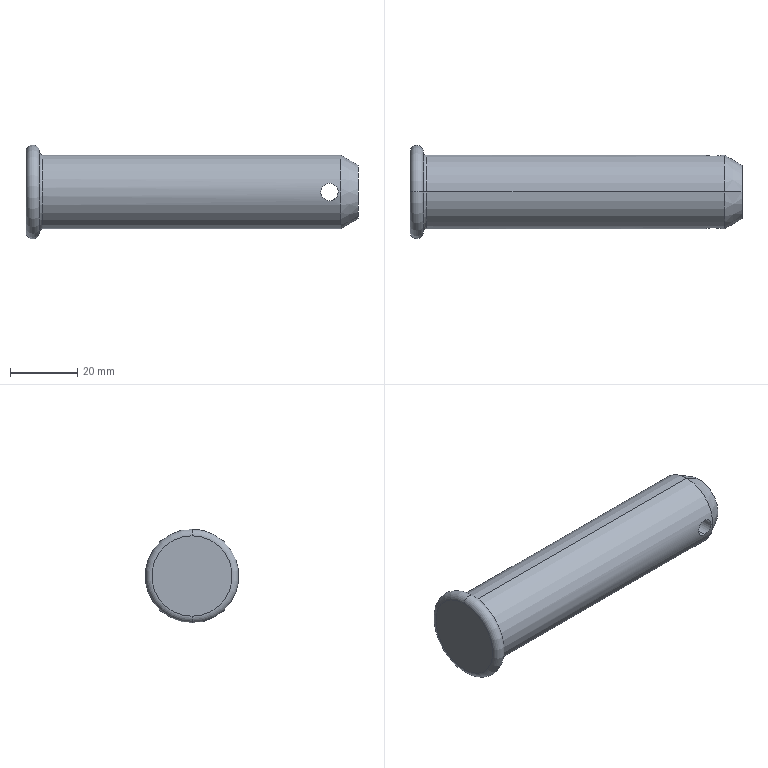Part | SolidWorks | features Chamfer 1, Cut 1, Fillet 1, Revolution 1 | 1 solid | 12 faces | box 99 x 28 x 28 mm | volume 37494 mm3 | cylinder 4 | torus 4 | cone 2 | plane 2 | commonest cylinder face diameters 5.18 x2 22 x2
STEP:
#1=CARTESIAN_POINT('',(90.5,-10.691,-2.59));
#2=VERTEX_POINT('',#1);
#3=CARTESIAN_POINT('',(90.5,-10.691,2.59));
#4=VERTEX_POINT('',#3);
#5=CARTESIAN_POINT('',(90.5,-10.691,-2.59));
#6=CARTESIAN_POINT('',(90.161,-10.691,-2.59));
#7=CARTESIAN_POINT('',(89.819,-10.708,-2.522));
#8=CARTESIAN_POINT('',(89.352,-10.751,-2.328));
#9=CARTESIAN_POINT('',(89.2,-10.769,-2.247));
#10=CARTESIAN_POINT('',(88.919,-10.806,-2.058));
#11=CARTESIAN_POINT('',(88.789,-10.826,-1.952));
#12=CARTESIAN_POINT('',(88.55,-10.866,-1.713));
#13=CARTESIAN_POINT('',(88.441,-10.887,-1.58));
#14=CARTESIAN_POINT('',(88.254,-10.924,-1.3));
#15=CARTESIAN_POINT('',(88.174,-10.941,-1.152));
#16=CARTESIAN_POINT('',(87.978,-10.984,-0.6798));
#17=CARTESIAN_POINT('',(87.91,-11.,-0.3427));
#18=CARTESIAN_POINT('',(87.91,-11.,0.1699));
#19=CARTESIAN_POINT('',(87.927,-10.996,0.3384));
#20=CARTESIAN_POINT('',(87.993,-10.981,0.6709));
#21=CARTESIAN_POINT('',(88.043,-10.969,0.8362));
#22=CARTESIAN_POINT('',(88.173,-10.941,1.149));
#23=CARTESIAN_POINT('',(88.252,-10.924,1.297));
#24=CARTESIAN_POINT('',(88.441,-10.887,1.58));
#25=CARTESIAN_POINT('',(88.549,-10.867,1.711));
#26=CARTESIAN_POINT('',(88.905,-10.806,2.068));
#27=CARTESIAN_POINT('',(89.193,-10.766,2.261));
#28=CARTESIAN_POINT('',(89.66,-10.723,2.456));
#29=CARTESIAN_POINT('',(89.825,-10.711,2.506));
#30=CARTESIAN_POINT('',(90.159,-10.695,2.573));
#31=CARTESIAN_POINT('',(90.328,-10.691,2.59));
#32=CARTESIAN_POINT('',(90.5,-10.691,2.59));
#33=B_SPLINE_CURVE_WITH_KNOTS('',3,(#5,#6,#7,#8,#9,#10,#11,#12,#13,#14,#15,#16,#17,#18,#19,#20,#21,#22,#23,#24,#25,#26,#27,#28,#29,#30,#31,#32),.UNSPECIFIED.,.F.,.F.,(4,2,2,2,2,2,2,2,2,2,2,2,2,4),(0.008126,0.009142,0.009649,0.01016,0.01066,0.01117,0.01219,0.0127,0.0132,0.01371,0.01422,0.01523,0.01574,0.01625),.UNSPECIFIED.);
#34=EDGE_CURVE('',#2,#4,#33,.T.);
#35=ORIENTED_EDGE('',*,*,#34,.F.);
#36=CARTESIAN_POINT('',(90.5,10.691,-2.59));
#37=VERTEX_POINT('',#36);
#38=CARTESIAN_POINT('',(90.5,-500.,-2.59));
#39=DIRECTION('',(0.,1.,0.));
#40=VECTOR('',#39,1000.);
#41=LINE('',#38,#40);
#42=EDGE_CURVE('',#2,#37,#41,.T.);
#43=ORIENTED_EDGE('',*,*,#42,.T.);
#44=CARTESIAN_POINT('',(90.5,10.691,2.59));
#45=VERTEX_POINT('',#44);
#46=CARTESIAN_POINT('',(90.5,10.691,2.59));
#47=CARTESIAN_POINT('',(90.328,10.691,2.59));
#48=CARTESIAN_POINT('',(90.159,10.695,2.573));
#49=CARTESIAN_POINT('',(89.828,10.711,2.507));
#50=CARTESIAN_POINT('',(89.663,10.722,2.457));
#51=CARTESIAN_POINT('',(89.349,10.751,2.327));
#52=CARTESIAN_POINT('',(89.201,10.768,2.247));
#53=CARTESIAN_POINT('',(88.92,10.806,2.059));
#54=CARTESIAN_POINT('',(88.787,10.826,1.95));
#55=CARTESIAN_POINT('',(88.43,10.887,1.593));
#56=CARTESIAN_POINT('',(88.237,10.927,1.305));
#57=CARTESIAN_POINT('',(88.043,10.969,0.8377));
#58=CARTESIAN_POINT('',(87.993,10.981,0.6738));
#59=CARTESIAN_POINT('',(87.927,10.996,0.3391));
#60=CARTESIAN_POINT('',(87.91,11.,0.1707));
#61=CARTESIAN_POINT('',(87.91,11.,-0.1686));
#62=CARTESIAN_POINT('',(87.927,10.996,-0.3409));
#63=CARTESIAN_POINT('',(87.993,10.981,-0.6736));
#64=CARTESIAN_POINT('',(88.043,10.969,-0.8353));
#65=CARTESIAN_POINT('',(88.238,10.927,-1.307));
#66=CARTESIAN_POINT('',(88.429,10.887,-1.592));
#67=CARTESIAN_POINT('',(88.789,10.826,-1.952));
#68=CARTESIAN_POINT('',(88.919,10.806,-2.059));
#69=CARTESIAN_POINT('',(89.199,10.769,-2.246));
#70=CARTESIAN_POINT('',(89.351,10.751,-2.327));
#71=CARTESIAN_POINT('',(89.664,10.722,-2.457));
#72=CARTESIAN_POINT('',(89.825,10.711,-2.506));
#73=CARTESIAN_POINT('',(90.159,10.695,-2.573));
#74=CARTESIAN_POINT('',(90.331,10.691,-2.59));
#75=CARTESIAN_POINT('',(90.5,10.691,-2.59));
#76=B_SPLINE_CURVE_WITH_KNOTS('',3,(#46,#47,#48,#49,#50,#51,#52,#53,#54,#55,#56,#57,#58,#59,#60,#61,#62,#63,#64,#65,#66,#67,#68,#69,#70,#71,#72,#73,#74,#75),.UNSPECIFIED.,.F.,.F.,(4,2,2,2,2,2,2,2,2,2,2,2,2,2,4),(0.,0.0005079,0.001016,0.001524,0.002032,0.003047,0.003555,0.004063,0.004571,0.005079,0.006095,0.006602,0.00711,0.007618,0.008126),.UNSPECIFIED.);
#77=EDGE_CURVE('',#45,#37,#76,.T.);
#78=ORIENTED_EDGE('',*,*,#77,.F.);
#79=CARTESIAN_POINT('',(90.5,-500.,2.59));
#80=DIRECTION('',(0.,1.,0.));
#81=VECTOR('',#80,1000.);
#82=LINE('',#79,#81);
#83=EDGE_CURVE('',#4,#45,#82,.T.);
#84=ORIENTED_EDGE('',*,*,#83,.F.);
#85=EDGE_LOOP('',(#35,#43,#78,#84));
#86=FACE_OUTER_BOUND('',#85,.T.);
#87=CARTESIAN_POINT('',(90.5,-500.,0.));
#88=DIRECTION('',(0.,1.,0.));
#89=DIRECTION('',(0.,0.,1.));
#90=AXIS2_PLACEMENT_3D('',#87,#88,#89);
#91=CYLINDRICAL_SURFACE('',#90,2.59);
#92=ADVANCED_FACE('',(#86),#91,.F.);
#93=CARTESIAN_POINT('',(99.,0.,-8.));
#94=VERTEX_POINT('',#93);
#95=CARTESIAN_POINT('',(99.,0.,8.));
#96=VERTEX_POINT('',#95);
#97=CARTESIAN_POINT('',(99.,0.,0.));
#98=DIRECTION('',(1.,0.,0.));
#99=DIRECTION('',(0.,0.,1.));
#100=AXIS2_PLACEMENT_3D('',#97,#98,#99);
#101=CIRCLE('',#100,8.);
#102=EDGE_CURVE('',#94,#96,#101,.T.);
#103=ORIENTED_EDGE('',*,*,#102,.F.);
#104=CARTESIAN_POINT('',(93.804,0.,-11.));
#105=VERTEX_POINT('',#104);
#106=CARTESIAN_POINT('',(93.804,0.,-11.));
#107=DIRECTION('',(-0.866,0.,-0.5));
#108=VECTOR('',#107,1000.);
#109=LINE('',#106,#108);
#110=EDGE_CURVE('',#94,#105,#109,.T.);
#111=ORIENTED_EDGE('',*,*,#110,.T.);
#112=CARTESIAN_POINT('',(93.804,0.,11.));
#113=VERTEX_POINT('',#112);
#114=CARTESIAN_POINT('',(93.804,0.,0.));
#115=DIRECTION('',(-1.,0.,0.));
#116=DIRECTION('',(0.,0.,1.));
#117=AXIS2_PLACEMENT_3D('',#114,#115,#116);
#118=CIRCLE('',#117,11.);
#119=EDGE_CURVE('',#113,#105,#118,.T.);
#120=ORIENTED_EDGE('',*,*,#119,.F.);
#121=CARTESIAN_POINT('',(93.804,0.,11.));
#122=DIRECTION('',(-0.866,0.,0.5));
#123=VECTOR('',#122,1000.);
#124=LINE('',#121,#123);
#125=EDGE_CURVE('',#96,#113,#124,.T.);
#126=ORIENTED_EDGE('',*,*,#125,.F.);
#127=EDGE_LOOP('',(#103,#111,#120,#126));
#128=FACE_OUTER_BOUND('',#127,.T.);
#129=CARTESIAN_POINT('',(93.804,0.,0.));
#130=DIRECTION('',(-1.,0.,0.));
#131=DIRECTION('',(0.,0.,1.));
#132=AXIS2_PLACEMENT_3D('',#129,#130,#131);
#133=CONICAL_SURFACE('',#132,11.,0.5236);
#134=ADVANCED_FACE('',(#128),#133,.T.);
#135=CARTESIAN_POINT('',(4.,0.,-12.));
#136=VERTEX_POINT('',#135);
#137=CARTESIAN_POINT('',(4.,0.,12.));
#138=VERTEX_POINT('',#137);
#139=CARTESIAN_POINT('',(4.,0.,0.));
#140=DIRECTION('',(-1.,0.,0.));
#141=DIRECTION('',(0.,0.,1.));
#142=AXIS2_PLACEMENT_3D('',#139,#140,#141);
#143=CIRCLE('',#142,12.);
#144=EDGE_CURVE('',#136,#138,#143,.T.);
#145=ORIENTED_EDGE('',*,*,#144,.F.);
#146=CARTESIAN_POINT('',(5.,0.,-11.));
#147=VERTEX_POINT('',#146);
#148=CARTESIAN_POINT('',(5.,0.,-12.));
#149=DIRECTION('',(0.,1.,0.));
#150=DIRECTION('',(0.,0.,1.));
#151=AXIS2_PLACEMENT_3D('',#148,#149,#150);
#152=CIRCLE('',#151,1.);
#153=EDGE_CURVE('',#136,#147,#152,.T.);
#154=ORIENTED_EDGE('',*,*,#153,.T.);
#155=CARTESIAN_POINT('',(5.,0.,11.));
#156=VERTEX_POINT('',#155);
#157=CARTESIAN_POINT('',(5.,0.,0.));
#158=DIRECTION('',(1.,0.,0.));
#159=DIRECTION('',(0.,0.,1.));
#160=AXIS2_PLACEMENT_3D('',#157,#158,#159);
#161=CIRCLE('',#160,11.);
#162=EDGE_CURVE('',#156,#147,#161,.T.);
#163=ORIENTED_EDGE('',*,*,#162,.F.);
#164=CARTESIAN_POINT('',(5.,0.,12.));
#165=DIRECTION('',(0.,-1.,0.));
#166=DIRECTION('',(0.,0.,-1.));
#167=AXIS2_PLACEMENT_3D('',#164,#165,#166);
#168=CIRCLE('',#167,1.);
#169=EDGE_CURVE('',#138,#156,#168,.T.);
#170=ORIENTED_EDGE('',*,*,#169,.F.);
#171=EDGE_LOOP('',(#145,#154,#163,#170));
#172=FACE_OUTER_BOUND('',#171,.T.);
#173=CARTESIAN_POINT('',(5.,0.,0.));
#174=DIRECTION('',(-1.,0.,0.));
#175=DIRECTION('',(0.,0.,1.));
#176=AXIS2_PLACEMENT_3D('',#173,#174,#175);
#177=TOROIDAL_SURFACE('',#176,12.,1.);
#178=ADVANCED_FACE('',(#172),#177,.F.);
#179=ORIENTED_EDGE('',*,*,#77,.T.);
#180=CARTESIAN_POINT('',(90.5,10.691,-2.59));
#181=CARTESIAN_POINT('',(90.839,10.691,-2.59));
#182=CARTESIAN_POINT('',(91.181,10.708,-2.522));
#183=CARTESIAN_POINT('',(91.648,10.751,-2.328));
#184=CARTESIAN_POINT('',(91.8,10.769,-2.247));
#185=CARTESIAN_POINT('',(92.081,10.806,-2.058));
#186=CARTESIAN_POINT('',(92.211,10.826,-1.952));
#187=CARTESIAN_POINT('',(92.45,10.866,-1.713));
#188=CARTESIAN_POINT('',(92.559,10.887,-1.58));
#189=CARTESIAN_POINT('',(92.746,10.924,-1.3));
#190=CARTESIAN_POINT('',(92.826,10.941,-1.152));
#191=CARTESIAN_POINT('',(93.022,10.984,-0.6798));
#192=CARTESIAN_POINT('',(93.09,11.,-0.3427));
#193=CARTESIAN_POINT('',(93.09,11.,0.1699));
#194=CARTESIAN_POINT('',(93.073,10.996,0.3384));
#195=CARTESIAN_POINT('',(93.007,10.981,0.6709));
#196=CARTESIAN_POINT('',(92.957,10.969,0.8362));
#197=CARTESIAN_POINT('',(92.827,10.941,1.149));
#198=CARTESIAN_POINT('',(92.748,10.924,1.297));
#199=CARTESIAN_POINT('',(92.559,10.887,1.58));
#200=CARTESIAN_POINT('',(92.451,10.867,1.711));
#201=CARTESIAN_POINT('',(92.095,10.806,2.068));
#202=CARTESIAN_POINT('',(91.807,10.766,2.261));
#203=CARTESIAN_POINT('',(91.34,10.723,2.456));
#204=CARTESIAN_POINT('',(91.175,10.711,2.506));
#205=CARTESIAN_POINT('',(90.841,10.695,2.573));
#206=CARTESIAN_POINT('',(90.672,10.691,2.59));
#207=CARTESIAN_POINT('',(90.5,10.691,2.59));
#208=B_SPLINE_CURVE_WITH_KNOTS('',3,(#180,#181,#182,#183,#184,#185,#186,#187,#188,#189,#190,#191,#192,#193,#194,#195,#196,#197,#198,#199,#200,#201,#202,#203,#204,#205,#206,#207),.UNSPECIFIED.,.F.,.F.,(4,2,2,2,2,2,2,2,2,2,2,2,2,4),(0.008126,0.009142,0.009649,0.01016,0.01066,0.01117,0.01219,0.0127,0.0132,0.01371,0.01422,0.01523,0.01574,0.01625),.UNSPECIFIED.);
#209=EDGE_CURVE('',#37,#45,#208,.T.);
#210=ORIENTED_EDGE('',*,*,#209,.T.);
#211=EDGE_LOOP('',(#179,#210));
#212=FACE_BOUND('',#211,.T.);
#213=ORIENTED_EDGE('',*,*,#119,.T.);
#214=CARTESIAN_POINT('',(0.,0.,-11.));
#215=DIRECTION('',(-1.,0.,0.));
#216=VECTOR('',#215,1000.);
#217=LINE('',#214,#216);
#218=EDGE_CURVE('',#105,#147,#217,.T.);
#219=ORIENTED_EDGE('',*,*,#218,.T.);
#220=CARTESIAN_POINT('',(5.,0.,0.));
#221=DIRECTION('',(1.,0.,0.));
#222=DIRECTION('',(0.,0.,1.));
#223=AXIS2_PLACEMENT_3D('',#220,#221,#222);
#224=CIRCLE('',#223,11.);
#225=EDGE_CURVE('',#147,#156,#224,.T.);
#226=ORIENTED_EDGE('',*,*,#225,.T.);
#227=CARTESIAN_POINT('',(0.,0.,11.));
#228=DIRECTION('',(-1.,0.,0.));
#229=VECTOR('',#228,1000.);
#230=LINE('',#227,#229);
#231=EDGE_CURVE('',#113,#156,#230,.T.);
#232=ORIENTED_EDGE('',*,*,#231,.F.);
#233=EDGE_LOOP('',(#213,#219,#226,#232));
#234=FACE_OUTER_BOUND('',#233,.T.);
#235=CARTESIAN_POINT('',(0.,0.,0.));
#236=DIRECTION('',(-1.,0.,0.));
#237=DIRECTION('',(0.,0.,1.));
#238=AXIS2_PLACEMENT_3D('',#235,#236,#237);
#239=CYLINDRICAL_SURFACE('',#238,11.);
#240=ADVANCED_FACE('',(#212,#234),#239,.T.);
#241=CARTESIAN_POINT('',(4.,0.,0.));
#242=DIRECTION('',(-1.,0.,0.));
#243=DIRECTION('',(0.,0.,1.));
#244=AXIS2_PLACEMENT_3D('',#241,#242,#243);
#245=CIRCLE('',#244,12.);
#246=EDGE_CURVE('',#138,#136,#245,.T.);
#247=ORIENTED_EDGE('',*,*,#246,.T.);
#248=CARTESIAN_POINT('',(0.,0.,-12.));
#249=VERTEX_POINT('',#248);
#250=CARTESIAN_POINT('',(2.,0.,-12.));
#251=DIRECTION('',(0.,1.,0.));
#252=DIRECTION('',(0.,0.,1.));
#253=AXIS2_PLACEMENT_3D('',#250,#251,#252);
#254=CIRCLE('',#253,2.);
#255=EDGE_CURVE('',#136,#249,#254,.T.);
#256=ORIENTED_EDGE('',*,*,#255,.T.);
#257=CARTESIAN_POINT('',(0.,0.,12.));
#258=VERTEX_POINT('',#257);
#259=CARTESIAN_POINT('',(0.,0.,0.));
#260=DIRECTION('',(-1.,0.,0.));
#261=DIRECTION('',(0.,0.,1.));
#262=AXIS2_PLACEMENT_3D('',#259,#260,#261);
#263=CIRCLE('',#262,12.);
#264=EDGE_CURVE('',#258,#249,#263,.T.);
#265=ORIENTED_EDGE('',*,*,#264,.F.);
#266=CARTESIAN_POINT('',(2.,0.,12.));
#267=DIRECTION('',(0.,-1.,0.));
#268=DIRECTION('',(0.,0.,-1.));
#269=AXIS2_PLACEMENT_3D('',#266,#267,#268);
#270=CIRCLE('',#269,2.);
#271=EDGE_CURVE('',#138,#258,#270,.T.);
#272=ORIENTED_EDGE('',*,*,#271,.F.);
#273=EDGE_LOOP('',(#247,#256,#265,#272));
#274=FACE_OUTER_BOUND('',#273,.T.);
#275=CARTESIAN_POINT('',(2.,0.,0.));
#276=DIRECTION('',(-1.,0.,0.));
#277=DIRECTION('',(0.,0.,1.));
#278=AXIS2_PLACEMENT_3D('',#275,#276,#277);
#279=TOROIDAL_SURFACE('',#278,12.,2.);
#280=ADVANCED_FACE('',(#274),#279,.T.);
#281=ORIENTED_EDGE('',*,*,#264,.T.);
#282=CARTESIAN_POINT('',(0.,0.,0.));
#283=DIRECTION('',(-1.,0.,0.));
#284=DIRECTION('',(0.,0.,1.));
#285=AXIS2_PLACEMENT_3D('',#282,#283,#284);
#286=CIRCLE('',#285,12.);
#287=EDGE_CURVE('',#249,#258,#286,.T.);
#288=ORIENTED_EDGE('',*,*,#287,.T.);
#289=EDGE_LOOP('',(#281,#288));
#290=FACE_OUTER_BOUND('',#289,.T.);
#291=CARTESIAN_POINT('',(0.,0.,0.));
#292=DIRECTION('',(1.,0.,0.));
#293=DIRECTION('',(0.,0.,-1.));
#294=AXIS2_PLACEMENT_3D('',#291,#292,#293);
#295=PLANE('',#294);
#296=ADVANCED_FACE('',(#290),#295,.F.);
#297=ORIENTED_EDGE('',*,*,#255,.F.);
#298=ORIENTED_EDGE('',*,*,#144,.T.);
#299=ORIENTED_EDGE('',*,*,#271,.T.);
#300=ORIENTED_EDGE('',*,*,#287,.F.);
#301=EDGE_LOOP('',(#297,#298,#299,#300));
#302=FACE_OUTER_BOUND('',#301,.T.);
#303=CARTESIAN_POINT('',(2.,0.,0.));
#304=DIRECTION('',(-1.,0.,0.));
#305=DIRECTION('',(0.,0.,1.));
#306=AXIS2_PLACEMENT_3D('',#303,#304,#305);
#307=TOROIDAL_SURFACE('',#306,12.,2.);
#308=ADVANCED_FACE('',(#302),#307,.T.);
#309=ORIENTED_EDGE('',*,*,#218,.F.);
#310=CARTESIAN_POINT('',(93.804,0.,0.));
#311=DIRECTION('',(-1.,0.,0.));
#312=DIRECTION('',(0.,0.,1.));
#313=AXIS2_PLACEMENT_3D('',#310,#311,#312);
#314=CIRCLE('',#313,11.);
#315=EDGE_CURVE('',#105,#113,#314,.T.);
#316=ORIENTED_EDGE('',*,*,#315,.T.);
#317=ORIENTED_EDGE('',*,*,#231,.T.);
#318=ORIENTED_EDGE('',*,*,#162,.T.);
#319=EDGE_LOOP('',(#309,#316,#317,#318));
#320=FACE_OUTER_BOUND('',#319,.T.);
#321=CARTESIAN_POINT('',(90.5,-10.691,2.59));
#322=CARTESIAN_POINT('',(90.672,-10.691,2.59));
#323=CARTESIAN_POINT('',(90.841,-10.695,2.573));
#324=CARTESIAN_POINT('',(91.172,-10.711,2.507));
#325=CARTESIAN_POINT('',(91.337,-10.722,2.457));
#326=CARTESIAN_POINT('',(91.651,-10.751,2.327));
#327=CARTESIAN_POINT('',(91.799,-10.768,2.247));
#328=CARTESIAN_POINT('',(92.08,-10.806,2.059));
#329=CARTESIAN_POINT('',(92.213,-10.826,1.95));
#330=CARTESIAN_POINT('',(92.57,-10.887,1.593));
#331=CARTESIAN_POINT('',(92.763,-10.927,1.305));
#332=CARTESIAN_POINT('',(92.957,-10.969,0.8377));
#333=CARTESIAN_POINT('',(93.007,-10.981,0.6738));
#334=CARTESIAN_POINT('',(93.073,-10.996,0.3391));
#335=CARTESIAN_POINT('',(93.09,-11.,0.1707));
#336=CARTESIAN_POINT('',(93.09,-11.,-0.1686));
#337=CARTESIAN_POINT('',(93.073,-10.996,-0.3409));
#338=CARTESIAN_POINT('',(93.007,-10.981,-0.6736));
#339=CARTESIAN_POINT('',(92.957,-10.969,-0.8353));
#340=CARTESIAN_POINT('',(92.762,-10.927,-1.307));
#341=CARTESIAN_POINT('',(92.571,-10.887,-1.592));
#342=CARTESIAN_POINT('',(92.211,-10.826,-1.952));
#343=CARTESIAN_POINT('',(92.081,-10.806,-2.059));
#344=CARTESIAN_POINT('',(91.801,-10.769,-2.246));
#345=CARTESIAN_POINT('',(91.649,-10.751,-2.327));
#346=CARTESIAN_POINT('',(91.336,-10.722,-2.457));
#347=CARTESIAN_POINT('',(91.175,-10.711,-2.506));
#348=CARTESIAN_POINT('',(90.841,-10.695,-2.573));
#349=CARTESIAN_POINT('',(90.669,-10.691,-2.59));
#350=CARTESIAN_POINT('',(90.5,-10.691,-2.59));
#351=B_SPLINE_CURVE_WITH_KNOTS('',3,(#321,#322,#323,#324,#325,#326,#327,#328,#329,#330,#331,#332,#333,#334,#335,#336,#337,#338,#339,#340,#341,#342,#343,#344,#345,#346,#347,#348,#349,#350),.UNSPECIFIED.,.F.,.F.,(4,2,2,2,2,2,2,2,2,2,2,2,2,2,4),(0.,0.0005079,0.001016,0.001524,0.002032,0.003047,0.003555,0.004063,0.004571,0.005079,0.006095,0.006602,0.00711,0.007618,0.008126),.UNSPECIFIED.);
#352=EDGE_CURVE('',#4,#2,#351,.T.);
#353=ORIENTED_EDGE('',*,*,#352,.T.);
#354=ORIENTED_EDGE('',*,*,#34,.T.);
#355=EDGE_LOOP('',(#353,#354));
#356=FACE_BOUND('',#355,.T.);
#357=CARTESIAN_POINT('',(0.,0.,0.));
#358=DIRECTION('',(-1.,0.,0.));
#359=DIRECTION('',(0.,0.,1.));
#360=AXIS2_PLACEMENT_3D('',#357,#358,#359);
#361=CYLINDRICAL_SURFACE('',#360,11.);
#362=ADVANCED_FACE('',(#320,#356),#361,.T.);
#363=CARTESIAN_POINT('',(99.,0.,0.));
#364=DIRECTION('',(1.,0.,0.));
#365=DIRECTION('',(0.,0.,1.));
#366=AXIS2_PLACEMENT_3D('',#363,#364,#365);
#367=CIRCLE('',#366,8.);
#368=EDGE_CURVE('',#96,#94,#367,.T.);
#369=ORIENTED_EDGE('',*,*,#368,.T.);
#370=ORIENTED_EDGE('',*,*,#102,.T.);
#371=EDGE_LOOP('',(#369,#370));
#372=FACE_OUTER_BOUND('',#371,.T.);
#373=CARTESIAN_POINT('',(99.,11.,0.));
#374=DIRECTION('',(-1.,0.,0.));
#375=DIRECTION('',(0.,0.,1.));
#376=AXIS2_PLACEMENT_3D('',#373,#374,#375);
#377=PLANE('',#376);
#378=ADVANCED_FACE('',(#372),#377,.F.);
#379=ORIENTED_EDGE('',*,*,#153,.F.);
#380=ORIENTED_EDGE('',*,*,#246,.F.);
#381=ORIENTED_EDGE('',*,*,#169,.T.);
#382=ORIENTED_EDGE('',*,*,#225,.F.);
#383=EDGE_LOOP('',(#379,#380,#381,#382));
#384=FACE_OUTER_BOUND('',#383,.T.);
#385=CARTESIAN_POINT('',(5.,0.,0.));
#386=DIRECTION('',(-1.,0.,0.));
#387=DIRECTION('',(0.,0.,1.));
#388=AXIS2_PLACEMENT_3D('',#385,#386,#387);
#389=TOROIDAL_SURFACE('',#388,12.,1.);
#390=ADVANCED_FACE('',(#384),#389,.F.);
#391=ORIENTED_EDGE('',*,*,#110,.F.);
#392=ORIENTED_EDGE('',*,*,#368,.F.);
#393=ORIENTED_EDGE('',*,*,#125,.T.);
#394=ORIENTED_EDGE('',*,*,#315,.F.);
#395=EDGE_LOOP('',(#391,#392,#393,#394));
#396=FACE_OUTER_BOUND('',#395,.T.);
#397=CARTESIAN_POINT('',(93.804,0.,0.));
#398=DIRECTION('',(-1.,0.,0.));
#399=DIRECTION('',(0.,0.,1.));
#400=AXIS2_PLACEMENT_3D('',#397,#398,#399);
#401=CONICAL_SURFACE('',#400,11.,0.5236);
#402=ADVANCED_FACE('',(#396),#401,.T.);
#403=ORIENTED_EDGE('',*,*,#42,.F.);
#404=ORIENTED_EDGE('',*,*,#352,.F.);
#405=ORIENTED_EDGE('',*,*,#83,.T.);
#406=ORIENTED_EDGE('',*,*,#209,.F.);
#407=EDGE_LOOP('',(#403,#404,#405,#406));
#408=FACE_OUTER_BOUND('',#407,.T.);
#409=CARTESIAN_POINT('',(90.5,-500.,0.));
#410=DIRECTION('',(0.,1.,0.));
#411=DIRECTION('',(0.,0.,1.));
#412=AXIS2_PLACEMENT_3D('',#409,#410,#411);
#413=CYLINDRICAL_SURFACE('',#412,2.59);
#414=ADVANCED_FACE('',(#408),#413,.F.);
#415=CLOSED_SHELL('',(#92,#134,#178,#240,#280,#296,#308,#362,#378,#390,#402,#414));
#416=MANIFOLD_SOLID_BREP('',#415);
#417=CARTESIAN_POINT('',(0.,0.,0.));
#418=DIRECTION('',(0.,0.,1.));
#419=DIRECTION('',(1.,0.,0.));
#420=AXIS2_PLACEMENT_3D('',#417,#418,#419);
#421=(LENGTH_UNIT()NAMED_UNIT(*)SI_UNIT(.MILLI.,.METRE.));
#422=UNCERTAINTY_MEASURE_WITH_UNIT(LENGTH_MEASURE(0.00001),#421,'','');
#423=(NAMED_UNIT(*)PLANE_ANGLE_UNIT()SI_UNIT($,.RADIAN.));
#424=(NAMED_UNIT(*)SI_UNIT($,.STERADIAN.)SOLID_ANGLE_UNIT());
#425=(GEOMETRIC_REPRESENTATION_CONTEXT(3)GLOBAL_UNCERTAINTY_ASSIGNED_CONTEXT((#422))GLOBAL_UNIT_ASSIGNED_CONTEXT((#421,#423,#424))REPRESENTATION_CONTEXT('',''));
#426=ADVANCED_BREP_SHAPE_REPRESENTATION('',(#416,#420),#425);